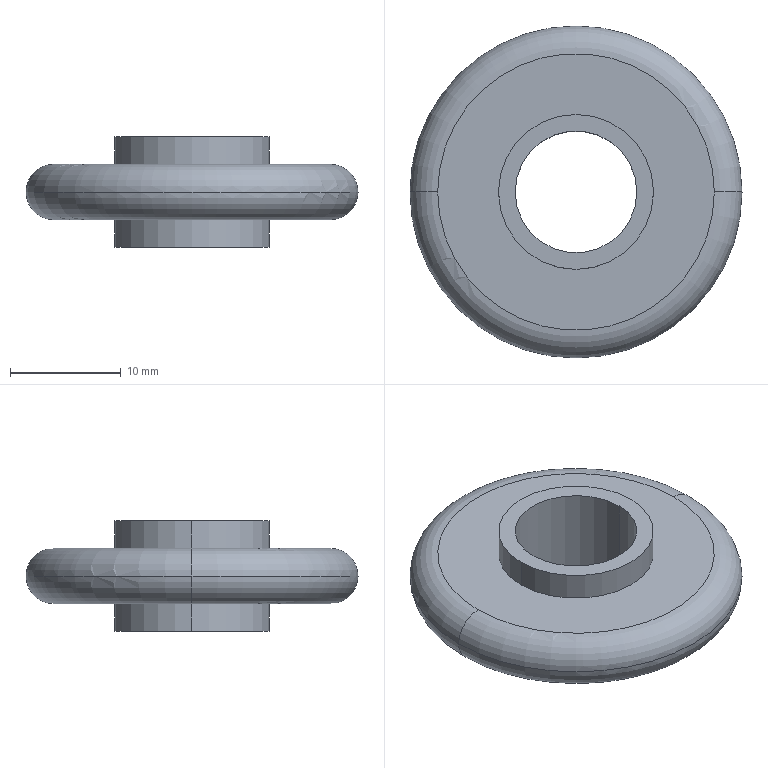Part | SolidWorks | features ICE 2, Extrusion 1, Fillet 1 | 1 solid | 14 faces | box 30 x 30 x 10 mm | volume 3110 mm3 | cylinder 6 | torus 4 | plane 4 | commonest cylinder face diameters 14 x4 11 x2
STEP:
#1=CARTESIAN_POINT('',(15.,0.,0.));
#2=VERTEX_POINT('',#1);
#3=CARTESIAN_POINT('',(-15.,0.,0.));
#4=VERTEX_POINT('',#3);
#5=CARTESIAN_POINT('',(0.,0.,0.));
#6=DIRECTION('',(0.,0.,1.));
#7=DIRECTION('',(1.,0.,0.));
#8=AXIS2_PLACEMENT_3D('',#5,#6,#7);
#9=CIRCLE('',#8,15.);
#10=EDGE_CURVE('',#2,#4,#9,.T.);
#11=ORIENTED_EDGE('',*,*,#10,.T.);
#12=CARTESIAN_POINT('',(-12.5,0.,2.5));
#13=VERTEX_POINT('',#12);
#14=CARTESIAN_POINT('',(-12.5,0.,0.));
#15=DIRECTION('',(0.,1.,0.));
#16=DIRECTION('',(-1.,0.,0.));
#17=AXIS2_PLACEMENT_3D('',#14,#15,#16);
#18=CIRCLE('',#17,2.5);
#19=EDGE_CURVE('',#4,#13,#18,.T.);
#20=ORIENTED_EDGE('',*,*,#19,.T.);
#21=CARTESIAN_POINT('',(12.5,0.,2.5));
#22=VERTEX_POINT('',#21);
#23=CARTESIAN_POINT('',(0.,0.,2.5));
#24=DIRECTION('',(0.,0.,1.));
#25=DIRECTION('',(1.,0.,0.));
#26=AXIS2_PLACEMENT_3D('',#23,#24,#25);
#27=CIRCLE('',#26,12.5);
#28=EDGE_CURVE('',#22,#13,#27,.T.);
#29=ORIENTED_EDGE('',*,*,#28,.F.);
#30=CARTESIAN_POINT('',(12.5,0.,0.));
#31=DIRECTION('',(0.,-1.,0.));
#32=DIRECTION('',(0.,0.,-1.));
#33=AXIS2_PLACEMENT_3D('',#30,#31,#32);
#34=CIRCLE('',#33,2.5);
#35=EDGE_CURVE('',#2,#22,#34,.T.);
#36=ORIENTED_EDGE('',*,*,#35,.F.);
#37=EDGE_LOOP('',(#11,#20,#29,#36));
#38=FACE_OUTER_BOUND('',#37,.T.);
#39=CARTESIAN_POINT('',(0.,0.,0.));
#40=DIRECTION('',(0.,0.,1.));
#41=DIRECTION('',(1.,0.,0.));
#42=AXIS2_PLACEMENT_3D('',#39,#40,#41);
#43=TOROIDAL_SURFACE('',#42,12.5,2.5);
#44=ADVANCED_FACE('',(#38),#43,.T.);
#45=CARTESIAN_POINT('',(-12.5,0.,-2.5));
#46=VERTEX_POINT('',#45);
#47=CARTESIAN_POINT('',(12.5,0.,-2.5));
#48=VERTEX_POINT('',#47);
#49=CARTESIAN_POINT('',(0.,0.,-2.5));
#50=DIRECTION('',(0.,0.,-1.));
#51=DIRECTION('',(1.,0.,0.));
#52=AXIS2_PLACEMENT_3D('',#49,#50,#51);
#53=CIRCLE('',#52,12.5);
#54=EDGE_CURVE('',#46,#48,#53,.T.);
#55=ORIENTED_EDGE('',*,*,#54,.F.);
#56=CARTESIAN_POINT('',(-12.5,0.,0.));
#57=DIRECTION('',(0.,1.,0.));
#58=DIRECTION('',(-1.,0.,0.));
#59=AXIS2_PLACEMENT_3D('',#56,#57,#58);
#60=CIRCLE('',#59,2.5);
#61=EDGE_CURVE('',#46,#4,#60,.T.);
#62=ORIENTED_EDGE('',*,*,#61,.T.);
#63=ORIENTED_EDGE('',*,*,#10,.F.);
#64=CARTESIAN_POINT('',(12.5,0.,0.));
#65=DIRECTION('',(0.,-1.,0.));
#66=DIRECTION('',(0.,0.,-1.));
#67=AXIS2_PLACEMENT_3D('',#64,#65,#66);
#68=CIRCLE('',#67,2.5);
#69=EDGE_CURVE('',#48,#2,#68,.T.);
#70=ORIENTED_EDGE('',*,*,#69,.F.);
#71=EDGE_LOOP('',(#55,#62,#63,#70));
#72=FACE_OUTER_BOUND('',#71,.T.);
#73=CARTESIAN_POINT('',(0.,0.,0.));
#74=DIRECTION('',(0.,0.,1.));
#75=DIRECTION('',(1.,0.,0.));
#76=AXIS2_PLACEMENT_3D('',#73,#74,#75);
#77=TOROIDAL_SURFACE('',#76,12.5,2.5);
#78=ADVANCED_FACE('',(#72),#77,.T.);
#79=CARTESIAN_POINT('',(-5.5,0.,-5.));
#80=VERTEX_POINT('',#79);
#81=CARTESIAN_POINT('',(5.5,0.,-5.));
#82=VERTEX_POINT('',#81);
#83=CARTESIAN_POINT('',(0.,0.,-5.));
#84=DIRECTION('',(0.,0.,1.));
#85=DIRECTION('',(1.,0.,0.));
#86=AXIS2_PLACEMENT_3D('',#83,#84,#85);
#87=CIRCLE('',#86,5.5);
#88=EDGE_CURVE('',#80,#82,#87,.T.);
#89=ORIENTED_EDGE('',*,*,#88,.F.);
#90=CARTESIAN_POINT('',(-5.5,0.,5.));
#91=VERTEX_POINT('',#90);
#92=CARTESIAN_POINT('',(-5.5,0.,-5.));
#93=DIRECTION('',(0.,0.,1.));
#94=VECTOR('',#93,1000.);
#95=LINE('',#92,#94);
#96=EDGE_CURVE('',#80,#91,#95,.T.);
#97=ORIENTED_EDGE('',*,*,#96,.T.);
#98=CARTESIAN_POINT('',(5.5,0.,5.));
#99=VERTEX_POINT('',#98);
#100=CARTESIAN_POINT('',(0.,0.,5.));
#101=DIRECTION('',(0.,0.,1.));
#102=DIRECTION('',(1.,0.,0.));
#103=AXIS2_PLACEMENT_3D('',#100,#101,#102);
#104=CIRCLE('',#103,5.5);
#105=EDGE_CURVE('',#91,#99,#104,.T.);
#106=ORIENTED_EDGE('',*,*,#105,.T.);
#107=CARTESIAN_POINT('',(5.5,0.,-5.));
#108=DIRECTION('',(0.,0.,1.));
#109=VECTOR('',#108,1000.);
#110=LINE('',#107,#109);
#111=EDGE_CURVE('',#82,#99,#110,.T.);
#112=ORIENTED_EDGE('',*,*,#111,.F.);
#113=EDGE_LOOP('',(#89,#97,#106,#112));
#114=FACE_OUTER_BOUND('',#113,.T.);
#115=CARTESIAN_POINT('',(0.,0.,-5.));
#116=DIRECTION('',(0.,0.,1.));
#117=DIRECTION('',(1.,0.,0.));
#118=AXIS2_PLACEMENT_3D('',#115,#116,#117);
#119=CYLINDRICAL_SURFACE('',#118,5.5);
#120=ADVANCED_FACE('',(#114),#119,.F.);
#121=CARTESIAN_POINT('',(7.,0.,2.5));
#122=VERTEX_POINT('',#121);
#123=CARTESIAN_POINT('',(-7.,0.,2.5));
#124=VERTEX_POINT('',#123);
#125=CARTESIAN_POINT('',(0.,0.,2.5));
#126=DIRECTION('',(0.,0.,1.));
#127=DIRECTION('',(1.,0.,0.));
#128=AXIS2_PLACEMENT_3D('',#125,#126,#127);
#129=CIRCLE('',#128,7.);
#130=EDGE_CURVE('',#122,#124,#129,.T.);
#131=ORIENTED_EDGE('',*,*,#130,.T.);
#132=CARTESIAN_POINT('',(-7.,0.,5.));
#133=VERTEX_POINT('',#132);
#134=CARTESIAN_POINT('',(-7.,0.,-5.));
#135=DIRECTION('',(0.,0.,1.));
#136=VECTOR('',#135,1000.);
#137=LINE('',#134,#136);
#138=EDGE_CURVE('',#124,#133,#137,.T.);
#139=ORIENTED_EDGE('',*,*,#138,.T.);
#140=CARTESIAN_POINT('',(7.,0.,5.));
#141=VERTEX_POINT('',#140);
#142=CARTESIAN_POINT('',(0.,0.,5.));
#143=DIRECTION('',(0.,0.,1.));
#144=DIRECTION('',(1.,0.,0.));
#145=AXIS2_PLACEMENT_3D('',#142,#143,#144);
#146=CIRCLE('',#145,7.);
#147=EDGE_CURVE('',#141,#133,#146,.T.);
#148=ORIENTED_EDGE('',*,*,#147,.F.);
#149=CARTESIAN_POINT('',(7.,0.,-5.));
#150=DIRECTION('',(0.,0.,1.));
#151=VECTOR('',#150,1000.);
#152=LINE('',#149,#151);
#153=EDGE_CURVE('',#122,#141,#152,.T.);
#154=ORIENTED_EDGE('',*,*,#153,.F.);
#155=EDGE_LOOP('',(#131,#139,#148,#154));
#156=FACE_OUTER_BOUND('',#155,.T.);
#157=CARTESIAN_POINT('',(0.,0.,-5.));
#158=DIRECTION('',(0.,0.,1.));
#159=DIRECTION('',(1.,0.,0.));
#160=AXIS2_PLACEMENT_3D('',#157,#158,#159);
#161=CYLINDRICAL_SURFACE('',#160,7.);
#162=ADVANCED_FACE('',(#156),#161,.T.);
#163=CARTESIAN_POINT('',(7.,0.,-5.));
#164=VERTEX_POINT('',#163);
#165=CARTESIAN_POINT('',(-7.,0.,-5.));
#166=VERTEX_POINT('',#165);
#167=CARTESIAN_POINT('',(0.,0.,-5.));
#168=DIRECTION('',(0.,0.,1.));
#169=DIRECTION('',(1.,0.,0.));
#170=AXIS2_PLACEMENT_3D('',#167,#168,#169);
#171=CIRCLE('',#170,7.);
#172=EDGE_CURVE('',#164,#166,#171,.T.);
#173=ORIENTED_EDGE('',*,*,#172,.T.);
#174=CARTESIAN_POINT('',(-7.,0.,-2.5));
#175=VERTEX_POINT('',#174);
#176=CARTESIAN_POINT('',(-7.,0.,-5.));
#177=DIRECTION('',(0.,0.,1.));
#178=VECTOR('',#177,1000.);
#179=LINE('',#176,#178);
#180=EDGE_CURVE('',#166,#175,#179,.T.);
#181=ORIENTED_EDGE('',*,*,#180,.T.);
#182=CARTESIAN_POINT('',(7.,0.,-2.5));
#183=VERTEX_POINT('',#182);
#184=CARTESIAN_POINT('',(0.,0.,-2.5));
#185=DIRECTION('',(0.,0.,1.));
#186=DIRECTION('',(1.,0.,0.));
#187=AXIS2_PLACEMENT_3D('',#184,#185,#186);
#188=CIRCLE('',#187,7.);
#189=EDGE_CURVE('',#183,#175,#188,.T.);
#190=ORIENTED_EDGE('',*,*,#189,.F.);
#191=CARTESIAN_POINT('',(7.,0.,-5.));
#192=DIRECTION('',(0.,0.,1.));
#193=VECTOR('',#192,1000.);
#194=LINE('',#191,#193);
#195=EDGE_CURVE('',#164,#183,#194,.T.);
#196=ORIENTED_EDGE('',*,*,#195,.F.);
#197=EDGE_LOOP('',(#173,#181,#190,#196));
#198=FACE_OUTER_BOUND('',#197,.T.);
#199=CARTESIAN_POINT('',(0.,0.,-5.));
#200=DIRECTION('',(0.,0.,1.));
#201=DIRECTION('',(1.,0.,0.));
#202=AXIS2_PLACEMENT_3D('',#199,#200,#201);
#203=CYLINDRICAL_SURFACE('',#202,7.);
#204=ADVANCED_FACE('',(#198),#203,.T.);
#205=ORIENTED_EDGE('',*,*,#28,.T.);
#206=CARTESIAN_POINT('',(0.,0.,2.5));
#207=DIRECTION('',(0.,0.,1.));
#208=DIRECTION('',(1.,0.,0.));
#209=AXIS2_PLACEMENT_3D('',#206,#207,#208);
#210=CIRCLE('',#209,12.5);
#211=EDGE_CURVE('',#13,#22,#210,.T.);
#212=ORIENTED_EDGE('',*,*,#211,.T.);
#213=EDGE_LOOP('',(#205,#212));
#214=FACE_OUTER_BOUND('',#213,.T.);
#215=ORIENTED_EDGE('',*,*,#130,.F.);
#216=CARTESIAN_POINT('',(0.,0.,2.5));
#217=DIRECTION('',(0.,0.,1.));
#218=DIRECTION('',(1.,0.,0.));
#219=AXIS2_PLACEMENT_3D('',#216,#217,#218);
#220=CIRCLE('',#219,7.);
#221=EDGE_CURVE('',#124,#122,#220,.T.);
#222=ORIENTED_EDGE('',*,*,#221,.F.);
#223=EDGE_LOOP('',(#215,#222));
#224=FACE_BOUND('',#223,.T.);
#225=CARTESIAN_POINT('',(0.,0.,2.5));
#226=DIRECTION('',(0.,0.,1.));
#227=DIRECTION('',(1.,0.,0.));
#228=AXIS2_PLACEMENT_3D('',#225,#226,#227);
#229=PLANE('',#228);
#230=ADVANCED_FACE('',(#214,#224),#229,.T.);
#231=CARTESIAN_POINT('',(0.,0.,-2.5));
#232=DIRECTION('',(0.,0.,-1.));
#233=DIRECTION('',(1.,0.,0.));
#234=AXIS2_PLACEMENT_3D('',#231,#232,#233);
#235=CIRCLE('',#234,12.5);
#236=EDGE_CURVE('',#48,#46,#235,.T.);
#237=ORIENTED_EDGE('',*,*,#236,.T.);
#238=ORIENTED_EDGE('',*,*,#54,.T.);
#239=EDGE_LOOP('',(#237,#238));
#240=FACE_OUTER_BOUND('',#239,.T.);
#241=ORIENTED_EDGE('',*,*,#189,.T.);
#242=CARTESIAN_POINT('',(0.,0.,-2.5));
#243=DIRECTION('',(0.,0.,1.));
#244=DIRECTION('',(1.,0.,0.));
#245=AXIS2_PLACEMENT_3D('',#242,#243,#244);
#246=CIRCLE('',#245,7.);
#247=EDGE_CURVE('',#175,#183,#246,.T.);
#248=ORIENTED_EDGE('',*,*,#247,.T.);
#249=EDGE_LOOP('',(#241,#248));
#250=FACE_BOUND('',#249,.T.);
#251=CARTESIAN_POINT('',(0.,0.,-2.5));
#252=DIRECTION('',(0.,0.,1.));
#253=DIRECTION('',(1.,0.,0.));
#254=AXIS2_PLACEMENT_3D('',#251,#252,#253);
#255=PLANE('',#254);
#256=ADVANCED_FACE('',(#240,#250),#255,.F.);
#257=CARTESIAN_POINT('',(0.,0.,-5.));
#258=DIRECTION('',(0.,0.,1.));
#259=DIRECTION('',(1.,0.,0.));
#260=AXIS2_PLACEMENT_3D('',#257,#258,#259);
#261=CIRCLE('',#260,5.5);
#262=EDGE_CURVE('',#82,#80,#261,.T.);
#263=ORIENTED_EDGE('',*,*,#262,.T.);
#264=ORIENTED_EDGE('',*,*,#88,.T.);
#265=EDGE_LOOP('',(#263,#264));
#266=FACE_BOUND('',#265,.T.);
#267=ORIENTED_EDGE('',*,*,#172,.F.);
#268=CARTESIAN_POINT('',(0.,0.,-5.));
#269=DIRECTION('',(0.,0.,1.));
#270=DIRECTION('',(1.,0.,0.));
#271=AXIS2_PLACEMENT_3D('',#268,#269,#270);
#272=CIRCLE('',#271,7.);
#273=EDGE_CURVE('',#166,#164,#272,.T.);
#274=ORIENTED_EDGE('',*,*,#273,.F.);
#275=EDGE_LOOP('',(#267,#274));
#276=FACE_OUTER_BOUND('',#275,.T.);
#277=CARTESIAN_POINT('',(0.,0.,-5.));
#278=DIRECTION('',(0.,0.,1.));
#279=DIRECTION('',(1.,0.,0.));
#280=AXIS2_PLACEMENT_3D('',#277,#278,#279);
#281=PLANE('',#280);
#282=ADVANCED_FACE('',(#266,#276),#281,.F.);
#283=ORIENTED_EDGE('',*,*,#180,.F.);
#284=ORIENTED_EDGE('',*,*,#273,.T.);
#285=ORIENTED_EDGE('',*,*,#195,.T.);
#286=ORIENTED_EDGE('',*,*,#247,.F.);
#287=EDGE_LOOP('',(#283,#284,#285,#286));
#288=FACE_OUTER_BOUND('',#287,.T.);
#289=CARTESIAN_POINT('',(0.,0.,-5.));
#290=DIRECTION('',(0.,0.,1.));
#291=DIRECTION('',(1.,0.,0.));
#292=AXIS2_PLACEMENT_3D('',#289,#290,#291);
#293=CYLINDRICAL_SURFACE('',#292,7.);
#294=ADVANCED_FACE('',(#288),#293,.T.);
#295=ORIENTED_EDGE('',*,*,#138,.F.);
#296=ORIENTED_EDGE('',*,*,#221,.T.);
#297=ORIENTED_EDGE('',*,*,#153,.T.);
#298=CARTESIAN_POINT('',(0.,0.,5.));
#299=DIRECTION('',(0.,0.,1.));
#300=DIRECTION('',(1.,0.,0.));
#301=AXIS2_PLACEMENT_3D('',#298,#299,#300);
#302=CIRCLE('',#301,7.);
#303=EDGE_CURVE('',#133,#141,#302,.T.);
#304=ORIENTED_EDGE('',*,*,#303,.F.);
#305=EDGE_LOOP('',(#295,#296,#297,#304));
#306=FACE_OUTER_BOUND('',#305,.T.);
#307=CARTESIAN_POINT('',(0.,0.,-5.));
#308=DIRECTION('',(0.,0.,1.));
#309=DIRECTION('',(1.,0.,0.));
#310=AXIS2_PLACEMENT_3D('',#307,#308,#309);
#311=CYLINDRICAL_SURFACE('',#310,7.);
#312=ADVANCED_FACE('',(#306),#311,.T.);
#313=CARTESIAN_POINT('',(0.,0.,5.));
#314=DIRECTION('',(0.,0.,1.));
#315=DIRECTION('',(1.,0.,0.));
#316=AXIS2_PLACEMENT_3D('',#313,#314,#315);
#317=CIRCLE('',#316,5.5);
#318=EDGE_CURVE('',#99,#91,#317,.T.);
#319=ORIENTED_EDGE('',*,*,#318,.F.);
#320=ORIENTED_EDGE('',*,*,#105,.F.);
#321=EDGE_LOOP('',(#319,#320));
#322=FACE_BOUND('',#321,.T.);
#323=ORIENTED_EDGE('',*,*,#147,.T.);
#324=ORIENTED_EDGE('',*,*,#303,.T.);
#325=EDGE_LOOP('',(#323,#324));
#326=FACE_OUTER_BOUND('',#325,.T.);
#327=CARTESIAN_POINT('',(0.,0.,5.));
#328=DIRECTION('',(0.,0.,1.));
#329=DIRECTION('',(1.,0.,0.));
#330=AXIS2_PLACEMENT_3D('',#327,#328,#329);
#331=PLANE('',#330);
#332=ADVANCED_FACE('',(#322,#326),#331,.T.);
#333=ORIENTED_EDGE('',*,*,#96,.F.);
#334=ORIENTED_EDGE('',*,*,#262,.F.);
#335=ORIENTED_EDGE('',*,*,#111,.T.);
#336=ORIENTED_EDGE('',*,*,#318,.T.);
#337=EDGE_LOOP('',(#333,#334,#335,#336));
#338=FACE_OUTER_BOUND('',#337,.T.);
#339=CARTESIAN_POINT('',(0.,0.,-5.));
#340=DIRECTION('',(0.,0.,1.));
#341=DIRECTION('',(1.,0.,0.));
#342=AXIS2_PLACEMENT_3D('',#339,#340,#341);
#343=CYLINDRICAL_SURFACE('',#342,5.5);
#344=ADVANCED_FACE('',(#338),#343,.F.);
#345=ORIENTED_EDGE('',*,*,#61,.F.);
#346=ORIENTED_EDGE('',*,*,#236,.F.);
#347=ORIENTED_EDGE('',*,*,#69,.T.);
#348=CARTESIAN_POINT('',(0.,0.,0.));
#349=DIRECTION('',(0.,0.,1.));
#350=DIRECTION('',(1.,0.,0.));
#351=AXIS2_PLACEMENT_3D('',#348,#349,#350);
#352=CIRCLE('',#351,15.);
#353=EDGE_CURVE('',#4,#2,#352,.T.);
#354=ORIENTED_EDGE('',*,*,#353,.F.);
#355=EDGE_LOOP('',(#345,#346,#347,#354));
#356=FACE_OUTER_BOUND('',#355,.T.);
#357=CARTESIAN_POINT('',(0.,0.,0.));
#358=DIRECTION('',(0.,0.,1.));
#359=DIRECTION('',(1.,0.,0.));
#360=AXIS2_PLACEMENT_3D('',#357,#358,#359);
#361=TOROIDAL_SURFACE('',#360,12.5,2.5);
#362=ADVANCED_FACE('',(#356),#361,.T.);
#363=ORIENTED_EDGE('',*,*,#19,.F.);
#364=ORIENTED_EDGE('',*,*,#353,.T.);
#365=ORIENTED_EDGE('',*,*,#35,.T.);
#366=ORIENTED_EDGE('',*,*,#211,.F.);
#367=EDGE_LOOP('',(#363,#364,#365,#366));
#368=FACE_OUTER_BOUND('',#367,.T.);
#369=CARTESIAN_POINT('',(0.,0.,0.));
#370=DIRECTION('',(0.,0.,1.));
#371=DIRECTION('',(1.,0.,0.));
#372=AXIS2_PLACEMENT_3D('',#369,#370,#371);
#373=TOROIDAL_SURFACE('',#372,12.5,2.5);
#374=ADVANCED_FACE('',(#368),#373,.T.);
#375=CLOSED_SHELL('',(#44,#78,#120,#162,#204,#230,#256,#282,#294,#312,#332,#344,#362,#374));
#376=MANIFOLD_SOLID_BREP('',#375);
#377=CARTESIAN_POINT('',(0.,0.,0.));
#378=DIRECTION('',(0.,0.,1.));
#379=DIRECTION('',(1.,0.,0.));
#380=AXIS2_PLACEMENT_3D('',#377,#378,#379);
#381=(LENGTH_UNIT()NAMED_UNIT(*)SI_UNIT(.MILLI.,.METRE.));
#382=UNCERTAINTY_MEASURE_WITH_UNIT(LENGTH_MEASURE(0.00001),#381,'','');
#383=(NAMED_UNIT(*)PLANE_ANGLE_UNIT()SI_UNIT($,.RADIAN.));
#384=(NAMED_UNIT(*)SI_UNIT($,.STERADIAN.)SOLID_ANGLE_UNIT());
#385=(GEOMETRIC_REPRESENTATION_CONTEXT(3)GLOBAL_UNCERTAINTY_ASSIGNED_CONTEXT((#382))GLOBAL_UNIT_ASSIGNED_CONTEXT((#381,#383,#384))REPRESENTATION_CONTEXT('',''));
#386=ADVANCED_BREP_SHAPE_REPRESENTATION('',(#376,#380),#385);